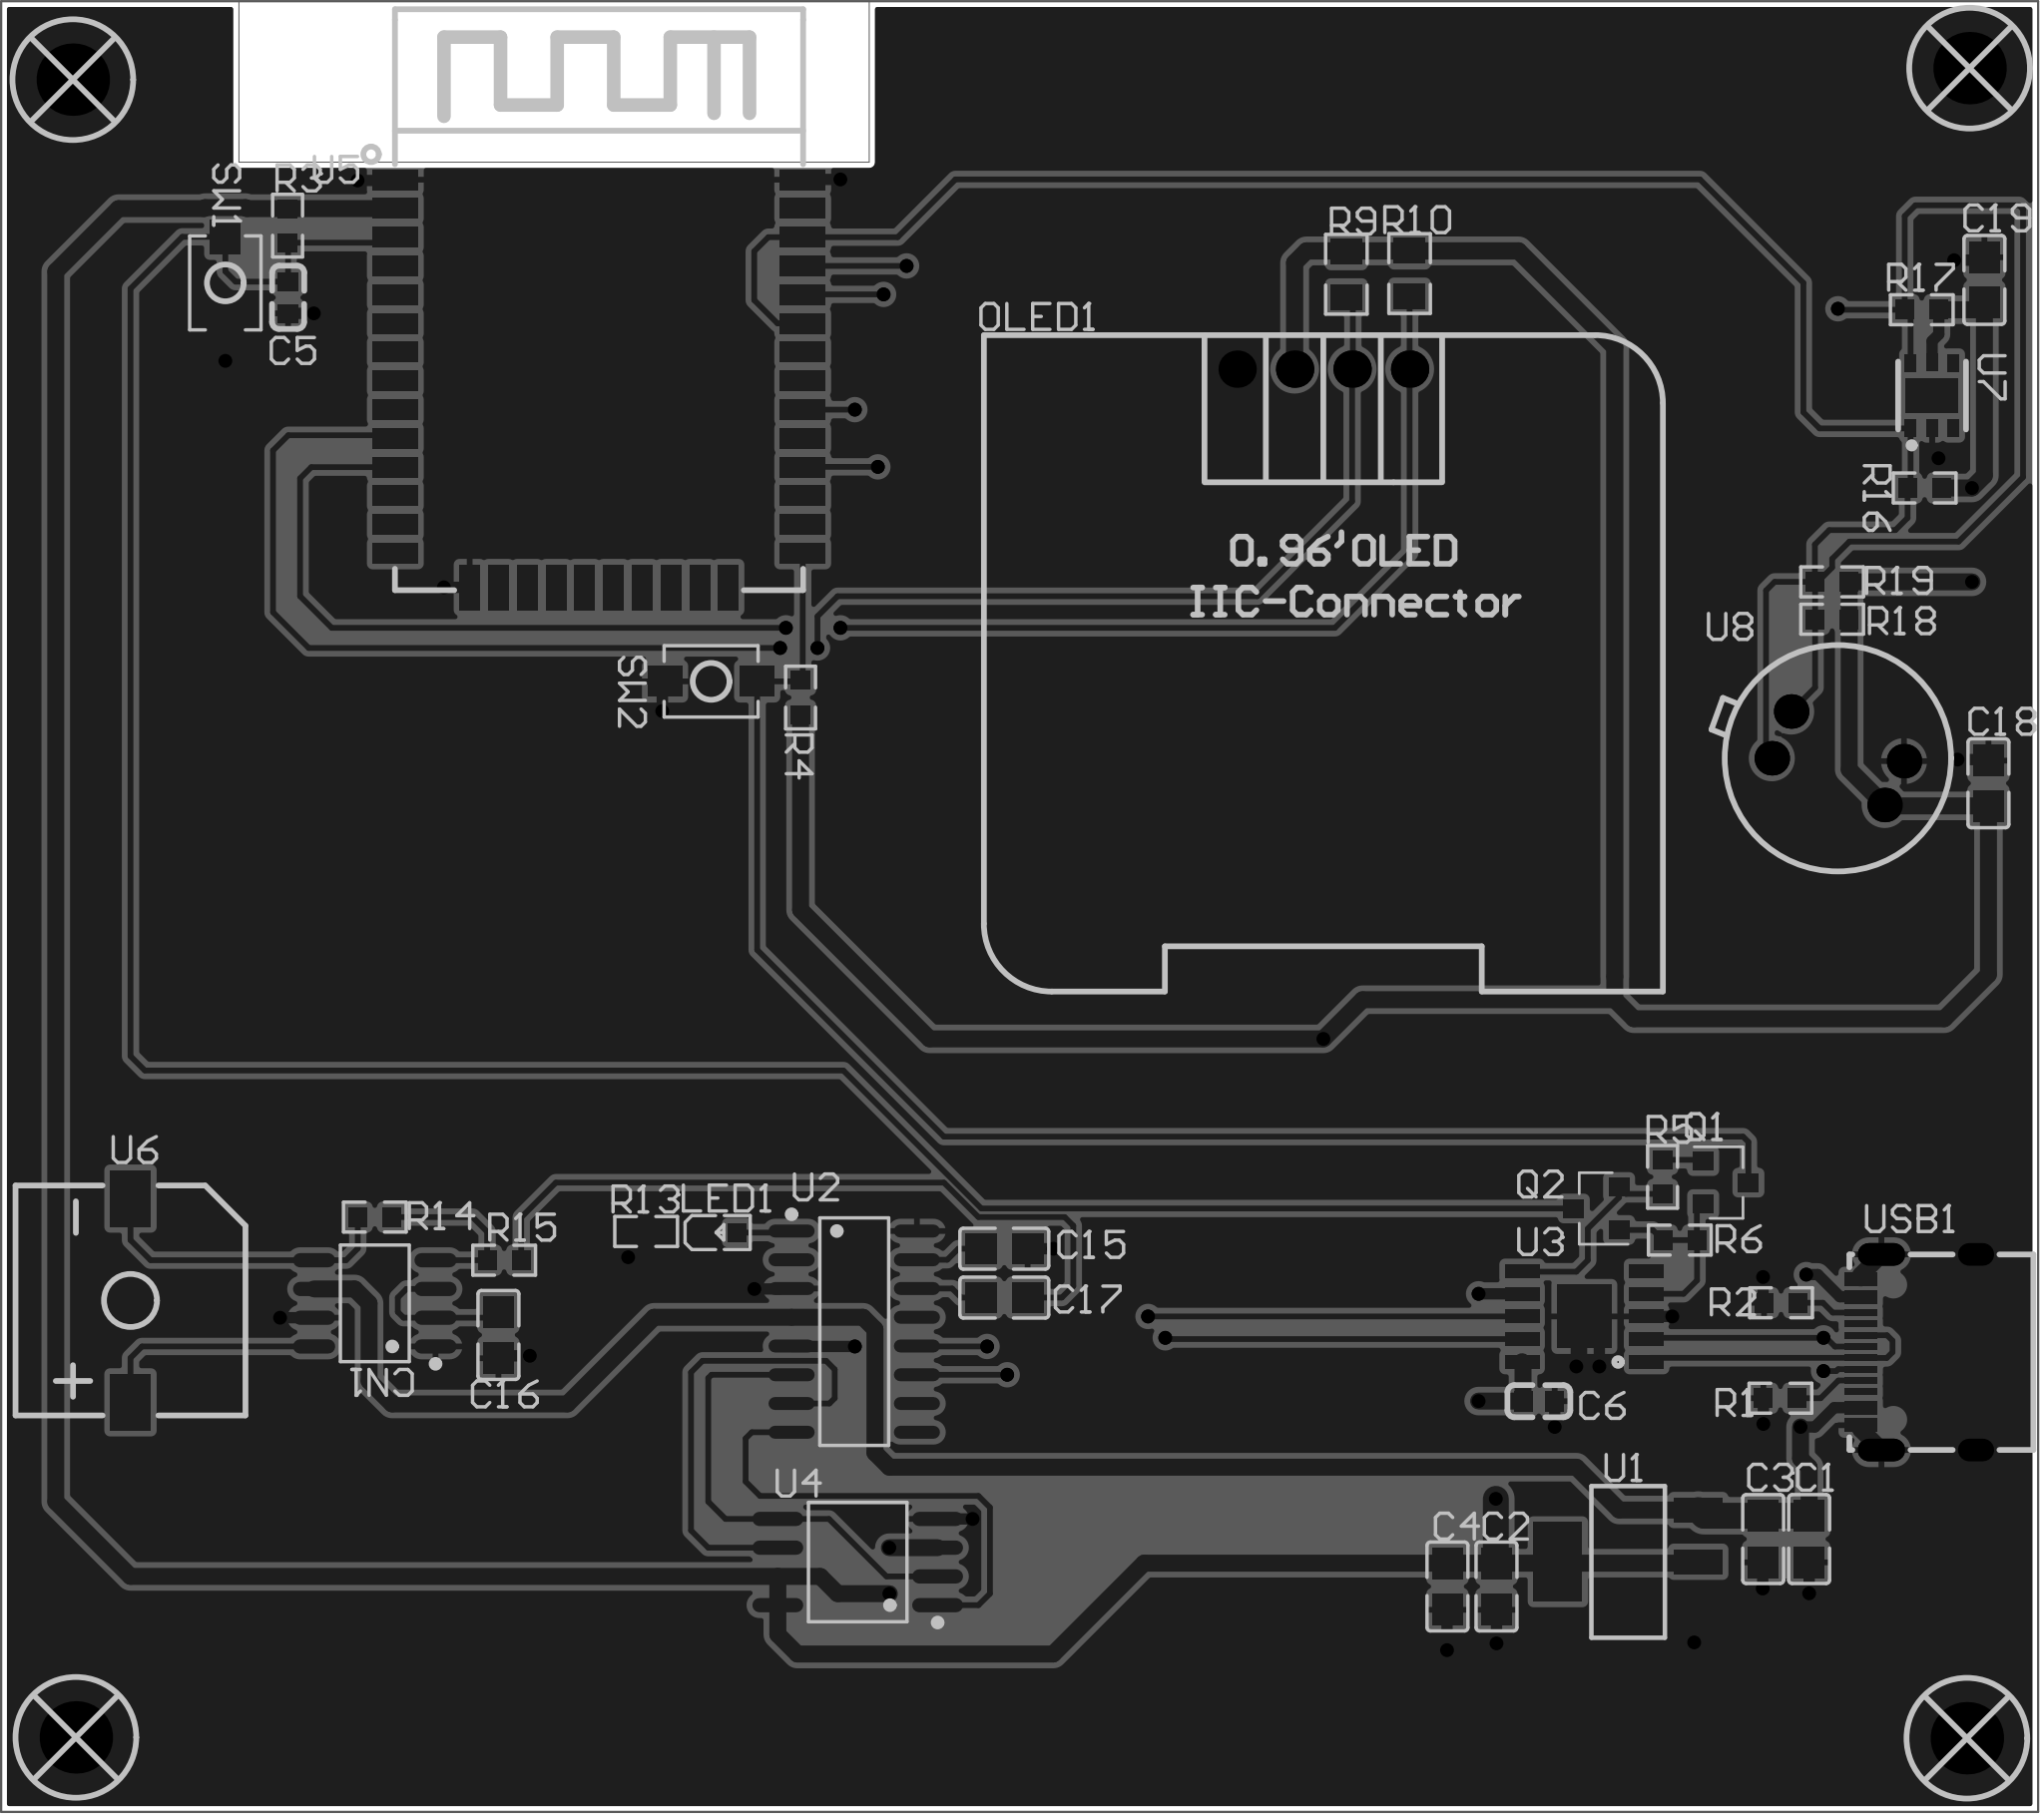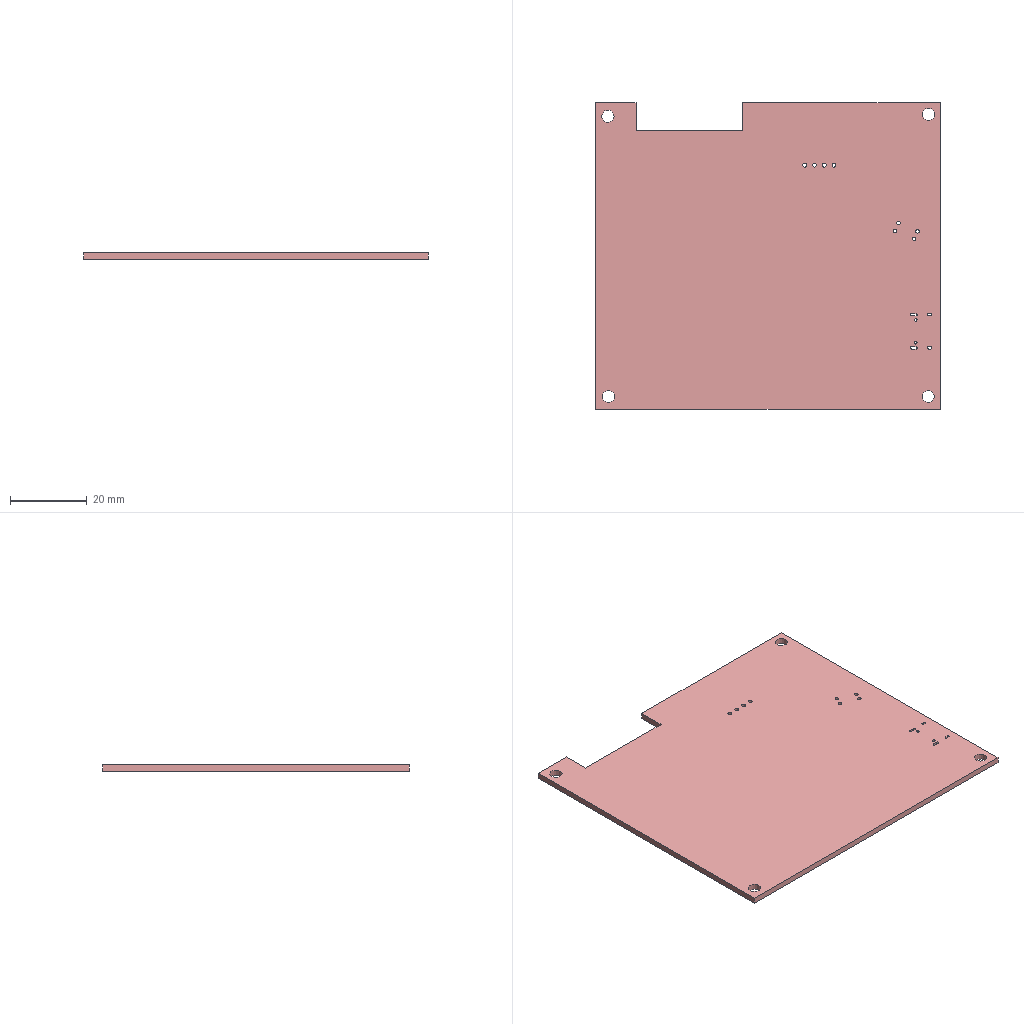Circuit board layout | Altium Designer | box 90 x 80 x 1.6 mm
Layer stack:
# Altium Designer layer stack of  (unit mm; dielectric type: 0 none, 1 core, 2 prepreg, 3 surface material)
index,name,kind,layer,copper_thickness_mm,dielectric_type,dielectric_thickness_mm,dielectric_material,dielectric_constant
0,Top Paste Mask Layer,other,,,,,,
1,Top Silkscreen Layer,other,,,,,,
2,Top Solder Mask Layer,dielectric,,,3,0.01,,3.3
3,Top Layer,copper,Top Layer,0.035,,,,
4,Dielectric1,dielectric,,,3,1.51,FR4,4.5
5,Bottom Layer,copper,Bottom Layer,0.035,,,,
6,Bottom Solder Mask Layer,dielectric,,,3,0.01,,3.3
7,Bottom Silkscreen Layer,other,,,,,,
8,Bottom Paste Mask Layer,other,,,,,,
# drill layer pairs: low layer,high layer
drill_pair,Top Layer,Bottom Layer
Part placement:
Designator,Comment,Layer,Footprint,Center-X(mm),Center-Y(mm),Rotation
C1,10u,TopLayer,C0805,164.084,101.854,90
C2,10u,TopLayer,C0805,150.27,99.758,90
C3,104,TopLayer,C0805,162.052,101.854,90
C4,104,TopLayer,C0805,148.104,99.758,90
C5,1uF,TopLayer,C0603,96.878,156.707,270
C6,100nF,TopLayer,C0603_1,152.142,107.945,180
C15,104,TopLayer,C0805,128.524,114.681,180
C16,105,TopLayer,C0805,106.172,110.871,270
C17,105,TopLayer,C0805,128.524,112.522,180
C18,22uF,TopLayer,C0805_1,172.006,135.245,270
C19,100nF,TopLayer,C0805_1,171.828,157.485,270
CN1,AD8002D,TopLayer,SOP-8_L5.0-W3.8-P1.27-LS6.0-BL,100.711,112.268,90
LED1,,TopLayer,LED_0603,115.908,115.391,0
Q1,S8050,TopLayer,SOT-23,160.401,117.602,0
Q2,S8050,TopLayer,SOT-23,154.686,116.459,180
R1,5.1kΩ,TopLayer,R0603,162.814,108.077,180
R2,5.1kΩ,TopLayer,R0603,162.843,112.293,180
R3,10kΩ,TopLayer,R0603,96.857,159.882,90
R4,10kΩ,TopLayer,R0603,119.523,139.033,270
R5,4.7kΩ,TopLayer,R0603,157.607,117.856,90
R6,4.7kΩ,TopLayer,R0603,158.369,115.062,180
R9,4.7K,TopLayer,R0805,143.637,157.734,270
R10,4.7K,TopLayer,R0805,146.431,157.766,270
R13,100R,TopLayer,R0603,112.699,115.443,0
R14,47K,TopLayer,R0603,100.711,116.078,180
R15,20K,TopLayer,R0603,106.426,114.173,180
R16,4.7K,TopLayer,R0603,169.186,148.292,0
R17,4.7K,TopLayer,R0603,169.059,156.166,0
R18,1.6K,TopLayer,R0603,165.1,142.494,0
R19,1.6K,TopLayer,R0603,165.1,144.145,0
SW1,,TopLayer,Key_SMD_3x4x2,94.107,157.353,270
SW2,,TopLayer,Key_SMD_3x4x2,115.569,139.747,180
U1,AMS1117-3.3,TopLayer,SOT-223_L6.5-W3.5-P2.30-LS7.0-BR,156.083,100.838,0
U2,JQ8400-FN,TopLayer,SOP-16_L9.9-W3.9-P1.27-LS6.0-BL,121.894,111.018,270
U3,CH340K,TopLayer,ESOP-10_L4.9-W3.9-P1.00-LS6.2-BL-EP,154.15,111.689,90
U4,W25Q128JVSIQ,TopLayer,SOIC-8_L5.3-W5.3-P1.27-LS8.0-BL,122.047,100.838,90
U5,2.4GHz,TopLayer,WIFIM-SMD_ESP32-WROOM-32-N4,110.617,152.908,0
U6,SPK-HN9650B,TopLayer,BUZ-SMD_L9.6-W9.6-LS10.0-R,89.916,112.395,270
U7,SHT20-TR-1.5KS,TopLayer,DFN-6_L3.0-W3.0-P0.95-TR-EP,169.515,152.376,180
U8,MLX90640ESF-BAA-000-TU,TopLayer,TO-39_4P-BD9.3_MLX90640ESF-BAA-000-TU_H5.7,165.354,136.351,0
USB1,,TopLayer,USB-C-SMD_TYPEC-304-BCP16,168.91,110.109,90
SCREW1,,TopLayer,M3螺丝,87.503,93.091,0
SCREW2,,TopLayer,M3螺丝,87.368,166.333,0
SCREW3,,TopLayer,M3螺丝,171.053,93.054,0
SCREW4,,TopLayer,M3螺丝,171.172,166.841,0
OLED1,,TopLayer,0.96OLED_4P,142.621,153.543,0
Pad and via stacks:
# Altium Designer via and pad stacks of  (unit mm). Each distinct definition once, with the count of objects using it.
# via: kind,start_layer,end_layer,hole_mm,diameter_mm,mode(0 simple;1 top-mid-bottom;2 full stack),diameter_per_layer,count,example_net
# pad: kind,layer,hole_mm,hole_type(0 round;1 square;2 slot),plating,top_size,top_shape(1 round;2 rect;3 octagon;9 rounded rect),mid_size,bottom_size,mode,footprint,size_per_layer,count,example
pad,Top Layer,0,0,plated,1.41x1.35,2,1.41x1.35,1.41x1.35,0,C0805,,14,C1.2
pad,Top Layer,0,0,plated,0.8x0.9,2,0.8x0.9,0.8x0.9,0,C0603,,2,C5.2
pad,Top Layer,0,0,plated,0.8x0.9,2,0.8x0.9,0.8x0.9,0,C0603_1,,2,C6.2
pad,Top Layer,0,0,plated,1.41x1.35,2,1.41x1.35,1.41x1.35,0,C0805_1,,4,C18.2
pad,Top Layer,0,0,plated,0.63x1.865,1,0.63x1.865,0.63x1.865,0,SOP-8_L5.0-W3.8-P1.27-LS6.0-BL,,8,CN1.5
pad,Top Layer,0,0,plated,0.8001x0.8001,2,0.8001x0.8001,0.8001x0.8001,0,LED_0603,,2,LED1.1
pad,Top Layer,0,0,plated,0.9x0.8,2,0.9x0.8,0.9x0.8,0,SOT-23,,6,Q1.1
pad,Top Layer,0,0,plated,0.8065x0.864,2,0.8065x0.864,0.8065x0.864,0,R0603,,26,R1.2
pad,Top Layer,0,0,plated,1.133x1.377,2,1.133x1.377,1.133x1.377,0,R0805,,4,R9.2
pad,Top Layer,0,0,plated,1.53x1.36,2,1.53x1.36,1.53x1.36,0,Key_SMD_3x4x2,,4,SW1.1
pad,Top Layer,0,0,plated,1.092x2.159,2,1.092x2.159,1.092x2.159,0,SOT-223_L6.5-W3.5-P2.30-LS7.0-BR,,3,U1.1
pad,Top Layer,0,0,plated,3.505x2.159,2,3.505x2.159,3.505x2.159,0,SOT-223_L6.5-W3.5-P2.30-LS7.0-BR,,1,U1.4
pad,Top Layer,0,0,plated,0.574x2.038,1,0.574x2.038,0.574x2.038,0,SOP-16_L9.9-W3.9-P1.27-LS6.0-BL,,16,U2.1
pad,Top Layer,0,0,plated,0.6x1.5,2,0.6x1.5,0.6x1.5,0,ESOP-10_L4.9-W3.9-P1.00-LS6.2-BL-EP,,10,U3.1
pad,Top Layer,0,0,plated,2.8x2.4,2,2.8x2.4,2.8x2.4,0,ESOP-10_L4.9-W3.9-P1.00-LS6.2-BL-EP,,1,U3.11
pad,Top Layer,0,0,plated,0.63x2.25,1,0.63x2.25,0.63x2.25,0,SOIC-8_L5.3-W5.3-P1.27-LS8.0-BL,,8,U4.1
pad,Top Layer,0,0,plated,2x0.9,2,2x0.9,2x0.9,0,WIFIM-SMD_ESP32-WROOM-32-N4,,38,U5.1
pad,Top Layer,0,0,plated,4.1x4.1,2,4.1x4.1,4.1x4.1,0,WIFIM-SMD_ESP32-WROOM-32-N4,,1,U5.39
pad,Top Layer,0,0,plated,2.5x1.8,2,2.5x1.8,2.5x1.8,0,BUZ-SMD_L9.6-W9.6-LS10.0-R,,2,U6.1
pad,Top Layer,0,0,plated,0.5x0.75,2,0.5x0.75,0.5x0.75,0,DFN-6_L3.0-W3.0-P0.95-TR-EP,,6,U7.1
pad,Top Layer,0,0,plated,1.5x2.3,2,1.5x2.3,1.5x2.3,0,DFN-6_L3.0-W3.0-P0.95-TR-EP,,1,U7.7
pad,Top Layer,0,0,plated,0.5994x1.45,2,0.5994x1.45,0.5994x1.45,0,USB-C-SMD_TYPEC-304-BCP16,,4,USB1.B1A12
pad,Top Layer,0,0,plated,0.2997x1.45,2,0.2997x1.45,0.2997x1.45,0,USB-C-SMD_TYPEC-304-BCP16,,8,USB1.B5
pad,Multi-Layer,0.9144,0,plated,1.524x1.524,1,1.524x1.524,1.524x1.524,0,TO-39_4P-BD9.3_MLX90640ESF-BAA-000-TU_H5.7,,4,U8.1
pad,Multi-Layer,0.5994,2,plated,1.001x1.6,1,1.001x1.6,1.001x1.6,0,USB-C-SMD_TYPEC-304-BCP16,,2,USB1.16
pad,Multi-Layer,0.5994,2,plated,1.001x2.101,1,1.001x2.101,1.001x2.101,0,USB-C-SMD_TYPEC-304-BCP16,,2,USB1.14
pad,Multi-Layer,3.2,0,plated,3.2x3.2,1,3.2x3.2,3.2x3.2,0,M3\u00C2\u00DD\u00CB\u00BF,,4,SCREW1.1
pad,Multi-Layer,1,0,plated,1.65x1.65,1,1.65x1.65,1.65x1.65,0,0.96OLED_4P,,4,OLED1.4
via,Top Layer,Bottom Layer,0.3048,0.61,0,,52,3V3
Copper pours:
name,layer,net,type(0 solid;1 hatched;2 none)
Top Layer-GND,Top Layer,GND,0
Bottom Layer-GND,Bottom Layer,GND,0